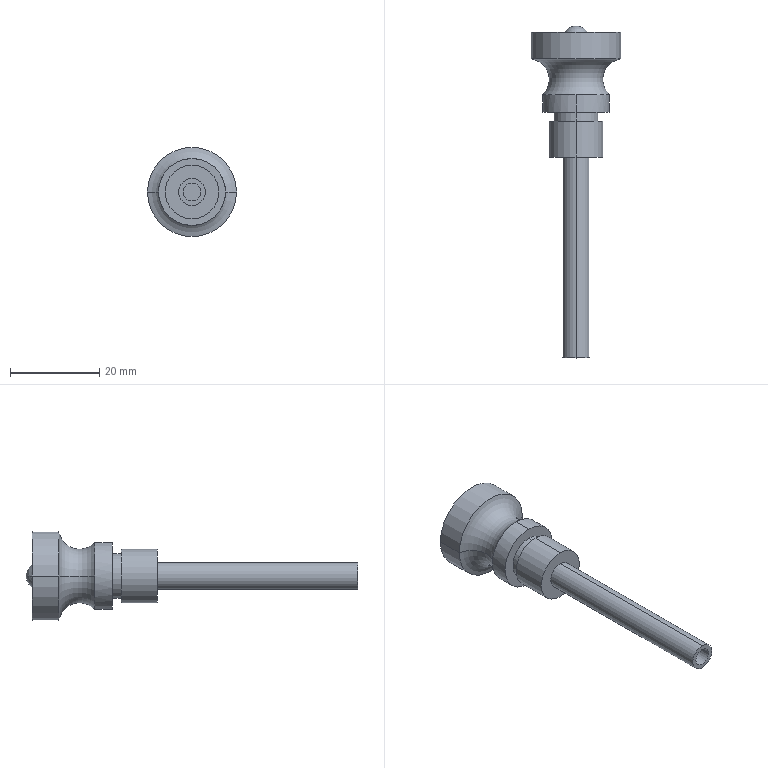Part | NX | features BREP 1 | 1 solid | 22 faces | box 20 x 74.367 x 20 mm | volume 5186 mm3 | cylinder 12 | plane 6 | torus 2 | sphere 2 | commonest cylinder face diameters 4 x2 6 x2 10 x2 12 x2 15 x2 20 x2
STEP:
#1=CARTESIAN_POINT('',(-10.,6.,0.));
#2=VERTEX_POINT('',#1);
#3=CARTESIAN_POINT('',(10.,6.,0.));
#4=VERTEX_POINT('',#3);
#5=CARTESIAN_POINT('',(0.,6.,0.));
#6=DIRECTION('',(0.,1.,0.));
#7=DIRECTION('',(-1.,0.,0.));
#8=AXIS2_PLACEMENT_3D('',#5,#6,#7);
#9=CIRCLE('',#8,10.);
#10=EDGE_CURVE('',#2,#4,#9,.T.);
#11=ORIENTED_EDGE('',*,*,#10,.T.);
#12=CARTESIAN_POINT('',(0.,6.,0.));
#13=DIRECTION('',(0.,1.,0.));
#14=DIRECTION('',(1.,0.,0.));
#15=AXIS2_PLACEMENT_3D('',#12,#13,#14);
#16=CIRCLE('',#15,10.);
#17=EDGE_CURVE('',#4,#2,#16,.T.);
#18=ORIENTED_EDGE('',*,*,#17,.T.);
#19=EDGE_LOOP('',(#11,#18));
#20=FACE_BOUND('',#19,.T.);
#21=CARTESIAN_POINT('',(-2.5,6.,0.));
#22=VERTEX_POINT('',#21);
#23=CARTESIAN_POINT('',(2.5,6.,0.));
#24=VERTEX_POINT('',#23);
#25=CARTESIAN_POINT('',(0.,6.,0.));
#26=DIRECTION('',(0.,-1.,0.));
#27=DIRECTION('',(-1.,0.,0.));
#28=AXIS2_PLACEMENT_3D('',#25,#26,#27);
#29=CIRCLE('',#28,2.5);
#30=EDGE_CURVE('',#22,#24,#29,.T.);
#31=ORIENTED_EDGE('',*,*,#30,.T.);
#32=CARTESIAN_POINT('',(0.,6.,0.));
#33=DIRECTION('',(0.,-1.,0.));
#34=DIRECTION('',(1.,0.,0.));
#35=AXIS2_PLACEMENT_3D('',#32,#33,#34);
#36=CIRCLE('',#35,2.5);
#37=EDGE_CURVE('',#24,#22,#36,.T.);
#38=ORIENTED_EDGE('',*,*,#37,.T.);
#39=EDGE_LOOP('',(#31,#38));
#40=FACE_BOUND('',#39,.T.);
#41=CARTESIAN_POINT('',(0.,6.,0.));
#42=DIRECTION('',(0.,1.,0.));
#43=DIRECTION('',(-1.,0.,0.));
#44=AXIS2_PLACEMENT_3D('',#41,#42,#43);
#45=PLANE('',#44);
#46=ADVANCED_FACE('',(#20,#40),#45,.T.);
#47=CARTESIAN_POINT('',(-10.,0.,0.));
#48=VERTEX_POINT('',#47);
#49=CARTESIAN_POINT('',(-10.,0.,0.));
#50=DIRECTION('',(0.,1.,0.));
#51=VECTOR('',#50,1000.);
#52=LINE('',#49,#51);
#53=EDGE_CURVE('',#48,#2,#52,.T.);
#54=ORIENTED_EDGE('',*,*,#53,.T.);
#55=ORIENTED_EDGE('',*,*,#17,.F.);
#56=CARTESIAN_POINT('',(10.,0.,0.));
#57=VERTEX_POINT('',#56);
#58=CARTESIAN_POINT('',(10.,0.,0.));
#59=DIRECTION('',(0.,1.,0.));
#60=VECTOR('',#59,1000.);
#61=LINE('',#58,#60);
#62=EDGE_CURVE('',#57,#4,#61,.T.);
#63=ORIENTED_EDGE('',*,*,#62,.F.);
#64=CARTESIAN_POINT('',(0.,0.,0.));
#65=DIRECTION('',(0.,-1.,0.));
#66=DIRECTION('',(-1.,0.,0.));
#67=AXIS2_PLACEMENT_3D('',#64,#65,#66);
#68=CIRCLE('',#67,10.);
#69=EDGE_CURVE('',#48,#57,#68,.T.);
#70=ORIENTED_EDGE('',*,*,#69,.F.);
#71=EDGE_LOOP('',(#54,#55,#63,#70));
#72=FACE_BOUND('',#71,.T.);
#73=CARTESIAN_POINT('',(0.,0.,0.));
#74=DIRECTION('',(0.,1.,0.));
#75=DIRECTION('',(-1.,0.,0.));
#76=AXIS2_PLACEMENT_3D('',#73,#74,#75);
#77=CYLINDRICAL_SURFACE('',#76,10.);
#78=ADVANCED_FACE('',(#72),#77,.T.);
#79=CARTESIAN_POINT('',(-7.5,-8.,0.));
#80=VERTEX_POINT('',#79);
#81=CARTESIAN_POINT('',(0.,-8.,-7.5));
#82=VERTEX_POINT('',#81);
#83=CARTESIAN_POINT('',(0.,-8.,0.));
#84=DIRECTION('',(0.,-1.,0.));
#85=DIRECTION('',(-1.,0.,0.));
#86=AXIS2_PLACEMENT_3D('',#83,#84,#85);
#87=CIRCLE('',#86,7.5);
#88=EDGE_CURVE('',#80,#82,#87,.T.);
#89=ORIENTED_EDGE('',*,*,#88,.F.);
#90=CARTESIAN_POINT('',(-10.631,-4.588,0.));
#91=DIRECTION('',(0.,0.,1.));
#92=DIRECTION('',(0.6761,-0.7368,0.));
#93=AXIS2_PLACEMENT_3D('',#90,#91,#92);
#94=CIRCLE('',#93,4.631);
#95=EDGE_CURVE('',#80,#48,#94,.T.);
#96=ORIENTED_EDGE('',*,*,#95,.T.);
#97=ORIENTED_EDGE('',*,*,#69,.T.);
#98=CARTESIAN_POINT('',(7.5,-8.,0.));
#99=VERTEX_POINT('',#98);
#100=CARTESIAN_POINT('',(10.631,-4.588,0.));
#101=DIRECTION('',(0.,0.,-1.));
#102=DIRECTION('',(-0.6761,-0.7368,0.));
#103=AXIS2_PLACEMENT_3D('',#100,#101,#102);
#104=CIRCLE('',#103,4.631);
#105=EDGE_CURVE('',#99,#57,#104,.T.);
#106=ORIENTED_EDGE('',*,*,#105,.F.);
#107=CARTESIAN_POINT('',(0.,-8.,0.));
#108=DIRECTION('',(0.,-1.,0.));
#109=DIRECTION('',(0.,0.,-1.));
#110=AXIS2_PLACEMENT_3D('',#107,#108,#109);
#111=CIRCLE('',#110,7.5);
#112=EDGE_CURVE('',#82,#99,#111,.T.);
#113=ORIENTED_EDGE('',*,*,#112,.F.);
#114=EDGE_LOOP('',(#89,#96,#97,#106,#113));
#115=FACE_BOUND('',#114,.T.);
#116=CARTESIAN_POINT('',(0.,-4.588,0.));
#117=DIRECTION('',(0.,-1.,0.));
#118=DIRECTION('',(1.,0.,0.));
#119=AXIS2_PLACEMENT_3D('',#116,#117,#118);
#120=TOROIDAL_SURFACE('',#119,10.631,4.631);
#121=ADVANCED_FACE('',(#115),#120,.F.);
#122=CARTESIAN_POINT('',(0.,-8.,7.5));
#123=VERTEX_POINT('',#122);
#124=CARTESIAN_POINT('',(0.,-8.,0.));
#125=DIRECTION('',(0.,-1.,0.));
#126=DIRECTION('',(1.,0.,0.));
#127=AXIS2_PLACEMENT_3D('',#124,#125,#126);
#128=CIRCLE('',#127,7.5);
#129=EDGE_CURVE('',#99,#123,#128,.T.);
#130=ORIENTED_EDGE('',*,*,#129,.T.);
#131=CARTESIAN_POINT('',(0.,-12.,7.5));
#132=VERTEX_POINT('',#131);
#133=CARTESIAN_POINT('',(0.,-8.,7.5));
#134=DIRECTION('',(0.,-1.,0.));
#135=VECTOR('',#134,1000.);
#136=LINE('',#133,#135);
#137=EDGE_CURVE('',#132,#123,#136,.F.);
#138=ORIENTED_EDGE('',*,*,#137,.F.);
#139=CARTESIAN_POINT('',(0.,-12.,-7.5));
#140=VERTEX_POINT('',#139);
#141=CARTESIAN_POINT('',(0.,-12.,0.));
#142=DIRECTION('',(0.,-1.,0.));
#143=DIRECTION('',(0.,0.,-1.));
#144=AXIS2_PLACEMENT_3D('',#141,#142,#143);
#145=CIRCLE('',#144,7.5);
#146=EDGE_CURVE('',#140,#132,#145,.T.);
#147=ORIENTED_EDGE('',*,*,#146,.F.);
#148=CARTESIAN_POINT('',(0.,-8.,-7.5));
#149=DIRECTION('',(0.,-1.,0.));
#150=VECTOR('',#149,1000.);
#151=LINE('',#148,#150);
#152=EDGE_CURVE('',#140,#82,#151,.F.);
#153=ORIENTED_EDGE('',*,*,#152,.T.);
#154=ORIENTED_EDGE('',*,*,#112,.T.);
#155=EDGE_LOOP('',(#130,#138,#147,#153,#154));
#156=FACE_BOUND('',#155,.T.);
#157=CARTESIAN_POINT('',(0.,-8.,0.));
#158=DIRECTION('',(0.,-1.,0.));
#159=DIRECTION('',(0.,0.,1.));
#160=AXIS2_PLACEMENT_3D('',#157,#158,#159);
#161=CYLINDRICAL_SURFACE('',#160,7.5);
#162=ADVANCED_FACE('',(#156),#161,.T.);
#163=ORIENTED_EDGE('',*,*,#88,.T.);
#164=ORIENTED_EDGE('',*,*,#152,.F.);
#165=CARTESIAN_POINT('',(0.,-12.,0.));
#166=DIRECTION('',(0.,-1.,0.));
#167=DIRECTION('',(0.,0.,1.));
#168=AXIS2_PLACEMENT_3D('',#165,#166,#167);
#169=CIRCLE('',#168,7.5);
#170=EDGE_CURVE('',#132,#140,#169,.T.);
#171=ORIENTED_EDGE('',*,*,#170,.F.);
#172=ORIENTED_EDGE('',*,*,#137,.T.);
#173=CARTESIAN_POINT('',(0.,-8.,0.));
#174=DIRECTION('',(0.,-1.,0.));
#175=DIRECTION('',(0.,0.,1.));
#176=AXIS2_PLACEMENT_3D('',#173,#174,#175);
#177=CIRCLE('',#176,7.5);
#178=EDGE_CURVE('',#123,#80,#177,.T.);
#179=ORIENTED_EDGE('',*,*,#178,.T.);
#180=EDGE_LOOP('',(#163,#164,#171,#172,#179));
#181=FACE_BOUND('',#180,.T.);
#182=CARTESIAN_POINT('',(0.,-8.,0.));
#183=DIRECTION('',(0.,-1.,0.));
#184=DIRECTION('',(0.,0.,1.));
#185=AXIS2_PLACEMENT_3D('',#182,#183,#184);
#186=CYLINDRICAL_SURFACE('',#185,7.5);
#187=ADVANCED_FACE('',(#181),#186,.T.);
#188=ORIENTED_EDGE('',*,*,#105,.T.);
#189=CARTESIAN_POINT('',(0.,0.,0.));
#190=DIRECTION('',(0.,-1.,0.));
#191=DIRECTION('',(1.,0.,0.));
#192=AXIS2_PLACEMENT_3D('',#189,#190,#191);
#193=CIRCLE('',#192,10.);
#194=EDGE_CURVE('',#57,#48,#193,.T.);
#195=ORIENTED_EDGE('',*,*,#194,.T.);
#196=ORIENTED_EDGE('',*,*,#95,.F.);
#197=ORIENTED_EDGE('',*,*,#178,.F.);
#198=ORIENTED_EDGE('',*,*,#129,.F.);
#199=EDGE_LOOP('',(#188,#195,#196,#197,#198));
#200=FACE_BOUND('',#199,.T.);
#201=CARTESIAN_POINT('',(0.,-4.588,0.));
#202=DIRECTION('',(0.,-1.,0.));
#203=DIRECTION('',(1.,0.,0.));
#204=AXIS2_PLACEMENT_3D('',#201,#202,#203);
#205=TOROIDAL_SURFACE('',#204,10.631,4.631);
#206=ADVANCED_FACE('',(#200),#205,.F.);
#207=ORIENTED_EDGE('',*,*,#62,.T.);
#208=ORIENTED_EDGE('',*,*,#10,.F.);
#209=ORIENTED_EDGE('',*,*,#53,.F.);
#210=ORIENTED_EDGE('',*,*,#194,.F.);
#211=EDGE_LOOP('',(#207,#208,#209,#210));
#212=FACE_BOUND('',#211,.T.);
#213=CARTESIAN_POINT('',(0.,0.,0.));
#214=DIRECTION('',(0.,1.,0.));
#215=DIRECTION('',(-1.,0.,0.));
#216=AXIS2_PLACEMENT_3D('',#213,#214,#215);
#217=CYLINDRICAL_SURFACE('',#216,10.);
#218=ADVANCED_FACE('',(#212),#217,.T.);
#219=ORIENTED_EDGE('',*,*,#170,.T.);
#220=ORIENTED_EDGE('',*,*,#146,.T.);
#221=EDGE_LOOP('',(#219,#220));
#222=FACE_BOUND('',#221,.T.);
#223=CARTESIAN_POINT('',(0.,-12.,5.));
#224=VERTEX_POINT('',#223);
#225=CARTESIAN_POINT('',(0.,-12.,-5.));
#226=VERTEX_POINT('',#225);
#227=CARTESIAN_POINT('',(0.,-12.,0.));
#228=DIRECTION('',(0.,-1.,0.));
#229=DIRECTION('',(0.,0.,1.));
#230=AXIS2_PLACEMENT_3D('',#227,#228,#229);
#231=CIRCLE('',#230,5.);
#232=EDGE_CURVE('',#224,#226,#231,.T.);
#233=ORIENTED_EDGE('',*,*,#232,.F.);
#234=CARTESIAN_POINT('',(0.,-12.,0.));
#235=DIRECTION('',(0.,-1.,0.));
#236=DIRECTION('',(0.,0.,-1.));
#237=AXIS2_PLACEMENT_3D('',#234,#235,#236);
#238=CIRCLE('',#237,5.);
#239=EDGE_CURVE('',#226,#224,#238,.T.);
#240=ORIENTED_EDGE('',*,*,#239,.F.);
#241=EDGE_LOOP('',(#233,#240));
#242=FACE_BOUND('',#241,.T.);
#243=CARTESIAN_POINT('',(0.,-12.,0.));
#244=DIRECTION('',(0.,-1.,0.));
#245=DIRECTION('',(0.,0.,1.));
#246=AXIS2_PLACEMENT_3D('',#243,#244,#245);
#247=PLANE('',#246);
#248=ADVANCED_FACE('',(#222,#242),#247,.T.);
#249=CARTESIAN_POINT('',(0.,-14.,-5.));
#250=VERTEX_POINT('',#249);
#251=CARTESIAN_POINT('',(0.,-12.,-5.));
#252=DIRECTION('',(0.,-1.,0.));
#253=VECTOR('',#252,1000.);
#254=LINE('',#251,#253);
#255=EDGE_CURVE('',#250,#226,#254,.F.);
#256=ORIENTED_EDGE('',*,*,#255,.T.);
#257=ORIENTED_EDGE('',*,*,#239,.T.);
#258=CARTESIAN_POINT('',(0.,-14.,5.));
#259=VERTEX_POINT('',#258);
#260=CARTESIAN_POINT('',(0.,-12.,5.));
#261=DIRECTION('',(0.,-1.,0.));
#262=VECTOR('',#261,1000.);
#263=LINE('',#260,#262);
#264=EDGE_CURVE('',#259,#224,#263,.F.);
#265=ORIENTED_EDGE('',*,*,#264,.F.);
#266=CARTESIAN_POINT('',(0.,-14.,0.));
#267=DIRECTION('',(0.,-1.,0.));
#268=DIRECTION('',(0.,0.,-1.));
#269=AXIS2_PLACEMENT_3D('',#266,#267,#268);
#270=CIRCLE('',#269,5.);
#271=EDGE_CURVE('',#250,#259,#270,.T.);
#272=ORIENTED_EDGE('',*,*,#271,.F.);
#273=EDGE_LOOP('',(#256,#257,#265,#272));
#274=FACE_BOUND('',#273,.T.);
#275=CARTESIAN_POINT('',(0.,-12.,0.));
#276=DIRECTION('',(0.,-1.,0.));
#277=DIRECTION('',(0.,0.,1.));
#278=AXIS2_PLACEMENT_3D('',#275,#276,#277);
#279=CYLINDRICAL_SURFACE('',#278,5.);
#280=ADVANCED_FACE('',(#274),#279,.T.);
#281=CARTESIAN_POINT('',(0.,-14.,6.));
#282=VERTEX_POINT('',#281);
#283=CARTESIAN_POINT('',(0.,-14.,-6.));
#284=VERTEX_POINT('',#283);
#285=CARTESIAN_POINT('',(0.,-14.,0.));
#286=DIRECTION('',(0.,-1.,0.));
#287=DIRECTION('',(0.,0.,1.));
#288=AXIS2_PLACEMENT_3D('',#285,#286,#287);
#289=CIRCLE('',#288,6.);
#290=EDGE_CURVE('',#282,#284,#289,.T.);
#291=ORIENTED_EDGE('',*,*,#290,.F.);
#292=CARTESIAN_POINT('',(0.,-14.,0.));
#293=DIRECTION('',(0.,-1.,0.));
#294=DIRECTION('',(0.,0.,-1.));
#295=AXIS2_PLACEMENT_3D('',#292,#293,#294);
#296=CIRCLE('',#295,6.);
#297=EDGE_CURVE('',#284,#282,#296,.T.);
#298=ORIENTED_EDGE('',*,*,#297,.F.);
#299=EDGE_LOOP('',(#291,#298));
#300=FACE_BOUND('',#299,.T.);
#301=CARTESIAN_POINT('',(0.,-14.,0.));
#302=DIRECTION('',(0.,-1.,0.));
#303=DIRECTION('',(0.,0.,1.));
#304=AXIS2_PLACEMENT_3D('',#301,#302,#303);
#305=CIRCLE('',#304,5.);
#306=EDGE_CURVE('',#259,#250,#305,.T.);
#307=ORIENTED_EDGE('',*,*,#306,.T.);
#308=ORIENTED_EDGE('',*,*,#271,.T.);
#309=EDGE_LOOP('',(#307,#308));
#310=FACE_BOUND('',#309,.T.);
#311=CARTESIAN_POINT('',(0.,-14.,0.));
#312=DIRECTION('',(0.,-1.,0.));
#313=DIRECTION('',(0.,0.,1.));
#314=AXIS2_PLACEMENT_3D('',#311,#312,#313);
#315=PLANE('',#314);
#316=ADVANCED_FACE('',(#300,#310),#315,.F.);
#317=CARTESIAN_POINT('',(0.,-22.,6.));
#318=VERTEX_POINT('',#317);
#319=CARTESIAN_POINT('',(0.,-14.,6.));
#320=DIRECTION('',(0.,-1.,0.));
#321=VECTOR('',#320,1000.);
#322=LINE('',#319,#321);
#323=EDGE_CURVE('',#318,#282,#322,.F.);
#324=ORIENTED_EDGE('',*,*,#323,.F.);
#325=CARTESIAN_POINT('',(0.,-22.,-6.));
#326=VERTEX_POINT('',#325);
#327=CARTESIAN_POINT('',(0.,-22.,0.));
#328=DIRECTION('',(0.,-1.,0.));
#329=DIRECTION('',(0.,0.,-1.));
#330=AXIS2_PLACEMENT_3D('',#327,#328,#329);
#331=CIRCLE('',#330,6.);
#332=EDGE_CURVE('',#326,#318,#331,.T.);
#333=ORIENTED_EDGE('',*,*,#332,.F.);
#334=CARTESIAN_POINT('',(0.,-14.,-6.));
#335=DIRECTION('',(0.,-1.,0.));
#336=VECTOR('',#335,1000.);
#337=LINE('',#334,#336);
#338=EDGE_CURVE('',#326,#284,#337,.F.);
#339=ORIENTED_EDGE('',*,*,#338,.T.);
#340=ORIENTED_EDGE('',*,*,#297,.T.);
#341=EDGE_LOOP('',(#324,#333,#339,#340));
#342=FACE_BOUND('',#341,.T.);
#343=CARTESIAN_POINT('',(0.,-14.,0.));
#344=DIRECTION('',(0.,-1.,0.));
#345=DIRECTION('',(0.,0.,1.));
#346=AXIS2_PLACEMENT_3D('',#343,#344,#345);
#347=CYLINDRICAL_SURFACE('',#346,6.);
#348=ADVANCED_FACE('',(#342),#347,.T.);
#349=ORIENTED_EDGE('',*,*,#338,.F.);
#350=CARTESIAN_POINT('',(0.,-22.,0.));
#351=DIRECTION('',(0.,-1.,0.));
#352=DIRECTION('',(0.,0.,1.));
#353=AXIS2_PLACEMENT_3D('',#350,#351,#352);
#354=CIRCLE('',#353,6.);
#355=EDGE_CURVE('',#318,#326,#354,.T.);
#356=ORIENTED_EDGE('',*,*,#355,.F.);
#357=ORIENTED_EDGE('',*,*,#323,.T.);
#358=ORIENTED_EDGE('',*,*,#290,.T.);
#359=EDGE_LOOP('',(#349,#356,#357,#358));
#360=FACE_BOUND('',#359,.T.);
#361=CARTESIAN_POINT('',(0.,-14.,0.));
#362=DIRECTION('',(0.,-1.,0.));
#363=DIRECTION('',(0.,0.,1.));
#364=AXIS2_PLACEMENT_3D('',#361,#362,#363);
#365=CYLINDRICAL_SURFACE('',#364,6.);
#366=ADVANCED_FACE('',(#360),#365,.T.);
#367=ORIENTED_EDGE('',*,*,#355,.T.);
#368=ORIENTED_EDGE('',*,*,#332,.T.);
#369=EDGE_LOOP('',(#367,#368));
#370=FACE_BOUND('',#369,.T.);
#371=CARTESIAN_POINT('',(0.,-22.,3.));
#372=VERTEX_POINT('',#371);
#373=CARTESIAN_POINT('',(0.,-22.,-3.));
#374=VERTEX_POINT('',#373);
#375=CARTESIAN_POINT('',(0.,-22.,0.));
#376=DIRECTION('',(0.,-1.,0.));
#377=DIRECTION('',(0.,0.,1.));
#378=AXIS2_PLACEMENT_3D('',#375,#376,#377);
#379=CIRCLE('',#378,3.);
#380=EDGE_CURVE('',#372,#374,#379,.T.);
#381=ORIENTED_EDGE('',*,*,#380,.F.);
#382=CARTESIAN_POINT('',(0.,-22.,0.));
#383=DIRECTION('',(0.,-1.,0.));
#384=DIRECTION('',(0.,0.,-1.));
#385=AXIS2_PLACEMENT_3D('',#382,#383,#384);
#386=CIRCLE('',#385,3.);
#387=EDGE_CURVE('',#374,#372,#386,.T.);
#388=ORIENTED_EDGE('',*,*,#387,.F.);
#389=EDGE_LOOP('',(#381,#388));
#390=FACE_BOUND('',#389,.T.);
#391=CARTESIAN_POINT('',(0.,-22.,0.));
#392=DIRECTION('',(0.,-1.,0.));
#393=DIRECTION('',(0.,0.,1.));
#394=AXIS2_PLACEMENT_3D('',#391,#392,#393);
#395=PLANE('',#394);
#396=ADVANCED_FACE('',(#370,#390),#395,.T.);
#397=CARTESIAN_POINT('',(0.,-67.,3.));
#398=VERTEX_POINT('',#397);
#399=CARTESIAN_POINT('',(0.,-22.,3.));
#400=DIRECTION('',(0.,-1.,0.));
#401=VECTOR('',#400,1000.);
#402=LINE('',#399,#401);
#403=EDGE_CURVE('',#398,#372,#402,.F.);
#404=ORIENTED_EDGE('',*,*,#403,.F.);
#405=CARTESIAN_POINT('',(0.,-67.,-3.));
#406=VERTEX_POINT('',#405);
#407=CARTESIAN_POINT('',(0.,-67.,0.));
#408=DIRECTION('',(0.,-1.,0.));
#409=DIRECTION('',(0.,0.,-1.));
#410=AXIS2_PLACEMENT_3D('',#407,#408,#409);
#411=CIRCLE('',#410,3.);
#412=EDGE_CURVE('',#406,#398,#411,.T.);
#413=ORIENTED_EDGE('',*,*,#412,.F.);
#414=CARTESIAN_POINT('',(0.,-22.,-3.));
#415=DIRECTION('',(0.,-1.,0.));
#416=VECTOR('',#415,1000.);
#417=LINE('',#414,#416);
#418=EDGE_CURVE('',#406,#374,#417,.F.);
#419=ORIENTED_EDGE('',*,*,#418,.T.);
#420=ORIENTED_EDGE('',*,*,#387,.T.);
#421=EDGE_LOOP('',(#404,#413,#419,#420));
#422=FACE_BOUND('',#421,.T.);
#423=CARTESIAN_POINT('',(0.,-22.,0.));
#424=DIRECTION('',(0.,-1.,0.));
#425=DIRECTION('',(0.,0.,1.));
#426=AXIS2_PLACEMENT_3D('',#423,#424,#425);
#427=CYLINDRICAL_SURFACE('',#426,3.);
#428=ADVANCED_FACE('',(#422),#427,.T.);
#429=ORIENTED_EDGE('',*,*,#418,.F.);
#430=CARTESIAN_POINT('',(0.,-67.,0.));
#431=DIRECTION('',(0.,-1.,0.));
#432=DIRECTION('',(0.,0.,1.));
#433=AXIS2_PLACEMENT_3D('',#430,#431,#432);
#434=CIRCLE('',#433,3.);
#435=EDGE_CURVE('',#398,#406,#434,.T.);
#436=ORIENTED_EDGE('',*,*,#435,.F.);
#437=ORIENTED_EDGE('',*,*,#403,.T.);
#438=ORIENTED_EDGE('',*,*,#380,.T.);
#439=EDGE_LOOP('',(#429,#436,#437,#438));
#440=FACE_BOUND('',#439,.T.);
#441=CARTESIAN_POINT('',(0.,-22.,0.));
#442=DIRECTION('',(0.,-1.,0.));
#443=DIRECTION('',(0.,0.,1.));
#444=AXIS2_PLACEMENT_3D('',#441,#442,#443);
#445=CYLINDRICAL_SURFACE('',#444,3.);
#446=ADVANCED_FACE('',(#440),#445,.T.);
#447=ORIENTED_EDGE('',*,*,#435,.T.);
#448=ORIENTED_EDGE('',*,*,#412,.T.);
#449=EDGE_LOOP('',(#447,#448));
#450=FACE_BOUND('',#449,.T.);
#451=CARTESIAN_POINT('',(2.,-67.,0.));
#452=VERTEX_POINT('',#451);
#453=CARTESIAN_POINT('',(-2.,-67.,0.));
#454=VERTEX_POINT('',#453);
#455=CARTESIAN_POINT('',(0.,-67.,0.));
#456=DIRECTION('',(0.,1.,0.));
#457=DIRECTION('',(1.,0.,0.));
#458=AXIS2_PLACEMENT_3D('',#455,#456,#457);
#459=CIRCLE('',#458,2.);
#460=EDGE_CURVE('',#452,#454,#459,.T.);
#461=ORIENTED_EDGE('',*,*,#460,.T.);
#462=CARTESIAN_POINT('',(0.,-67.,0.));
#463=DIRECTION('',(0.,1.,0.));
#464=DIRECTION('',(-1.,0.,0.));
#465=AXIS2_PLACEMENT_3D('',#462,#463,#464);
#466=CIRCLE('',#465,2.);
#467=EDGE_CURVE('',#454,#452,#466,.T.);
#468=ORIENTED_EDGE('',*,*,#467,.T.);
#469=EDGE_LOOP('',(#461,#468));
#470=FACE_BOUND('',#469,.T.);
#471=CARTESIAN_POINT('',(0.,-67.,0.));
#472=DIRECTION('',(0.,-1.,0.));
#473=DIRECTION('',(0.,0.,1.));
#474=AXIS2_PLACEMENT_3D('',#471,#472,#473);
#475=PLANE('',#474);
#476=ADVANCED_FACE('',(#450,#470),#475,.T.);
#477=CARTESIAN_POINT('',(2.,6.,0.));
#478=VERTEX_POINT('',#477);
#479=CARTESIAN_POINT('',(2.,-67.,0.));
#480=DIRECTION('',(0.,1.,0.));
#481=VECTOR('',#480,1000.);
#482=LINE('',#479,#481);
#483=EDGE_CURVE('',#452,#478,#482,.T.);
#484=ORIENTED_EDGE('',*,*,#483,.F.);
#485=ORIENTED_EDGE('',*,*,#467,.F.);
#486=CARTESIAN_POINT('',(-2.,6.,0.));
#487=VERTEX_POINT('',#486);
#488=CARTESIAN_POINT('',(-2.,-67.,0.));
#489=DIRECTION('',(0.,1.,0.));
#490=VECTOR('',#489,1000.);
#491=LINE('',#488,#490);
#492=EDGE_CURVE('',#454,#487,#491,.T.);
#493=ORIENTED_EDGE('',*,*,#492,.T.);
#494=CARTESIAN_POINT('',(0.,6.,0.));
#495=DIRECTION('',(0.,1.,0.));
#496=DIRECTION('',(-1.,0.,0.));
#497=AXIS2_PLACEMENT_3D('',#494,#495,#496);
#498=CIRCLE('',#497,2.);
#499=EDGE_CURVE('',#487,#478,#498,.T.);
#500=ORIENTED_EDGE('',*,*,#499,.T.);
#501=EDGE_LOOP('',(#484,#485,#493,#500));
#502=FACE_BOUND('',#501,.T.);
#503=CARTESIAN_POINT('',(0.,-67.,0.));
#504=DIRECTION('',(0.,1.,0.));
#505=DIRECTION('',(1.,0.,0.));
#506=AXIS2_PLACEMENT_3D('',#503,#504,#505);
#507=CYLINDRICAL_SURFACE('',#506,2.);
#508=ADVANCED_FACE('',(#502),#507,.F.);
#509=CARTESIAN_POINT('',(0.,6.,0.));
#510=DIRECTION('',(0.,1.,0.));
#511=DIRECTION('',(1.,0.,0.));
#512=AXIS2_PLACEMENT_3D('',#509,#510,#511);
#513=CIRCLE('',#512,2.);
#514=EDGE_CURVE('',#478,#487,#513,.T.);
#515=ORIENTED_EDGE('',*,*,#514,.F.);
#516=ORIENTED_EDGE('',*,*,#499,.F.);
#517=EDGE_LOOP('',(#515,#516));
#518=FACE_BOUND('',#517,.T.);
#519=CARTESIAN_POINT('',(0.,6.,0.));
#520=DIRECTION('',(0.,-1.,0.));
#521=DIRECTION('',(1.,0.,0.));
#522=AXIS2_PLACEMENT_3D('',#519,#520,#521);
#523=PLANE('',#522);
#524=ADVANCED_FACE('',(#518),#523,.T.);
#525=ORIENTED_EDGE('',*,*,#492,.F.);
#526=ORIENTED_EDGE('',*,*,#460,.F.);
#527=ORIENTED_EDGE('',*,*,#483,.T.);
#528=ORIENTED_EDGE('',*,*,#514,.T.);
#529=EDGE_LOOP('',(#525,#526,#527,#528));
#530=FACE_BOUND('',#529,.T.);
#531=CARTESIAN_POINT('',(0.,-67.,0.));
#532=DIRECTION('',(0.,1.,0.));
#533=DIRECTION('',(1.,0.,0.));
#534=AXIS2_PLACEMENT_3D('',#531,#532,#533);
#535=CYLINDRICAL_SURFACE('',#534,2.);
#536=ADVANCED_FACE('',(#530),#535,.F.);
#537=ORIENTED_EDGE('',*,*,#264,.T.);
#538=ORIENTED_EDGE('',*,*,#232,.T.);
#539=ORIENTED_EDGE('',*,*,#255,.F.);
#540=ORIENTED_EDGE('',*,*,#306,.F.);
#541=EDGE_LOOP('',(#537,#538,#539,#540));
#542=FACE_BOUND('',#541,.T.);
#543=CARTESIAN_POINT('',(0.,-12.,0.));
#544=DIRECTION('',(0.,-1.,0.));
#545=DIRECTION('',(0.,0.,1.));
#546=AXIS2_PLACEMENT_3D('',#543,#544,#545);
#547=CYLINDRICAL_SURFACE('',#546,5.);
#548=ADVANCED_FACE('',(#542),#547,.T.);
#549=CARTESIAN_POINT('',(0.,7.367,0.));
#550=VERTEX_POINT('',#549);
#551=CARTESIAN_POINT('',(0.,4.398,0.));
#552=DIRECTION('',(0.,0.,1.));
#553=DIRECTION('',(0.8419,0.5396,0.));
#554=AXIS2_PLACEMENT_3D('',#551,#552,#553);
#555=CIRCLE('',#554,2.969);
#556=EDGE_CURVE('',#550,#24,#555,.F.);
#557=ORIENTED_EDGE('',*,*,#556,.F.);
#558=CARTESIAN_POINT('',(0.,4.398,0.));
#559=DIRECTION('',(0.,0.,-1.));
#560=DIRECTION('',(-0.8419,0.5396,0.));
#561=AXIS2_PLACEMENT_3D('',#558,#559,#560);
#562=CIRCLE('',#561,2.969);
#563=EDGE_CURVE('',#550,#22,#562,.F.);
#564=ORIENTED_EDGE('',*,*,#563,.T.);
#565=ORIENTED_EDGE('',*,*,#37,.F.);
#566=EDGE_LOOP('',(#557,#564,#565));
#567=FACE_BOUND('',#566,.T.);
#568=CARTESIAN_POINT('',(0.,4.398,0.));
#569=DIRECTION('',(0.,-1.,0.));
#570=DIRECTION('',(1.,0.,0.));
#571=AXIS2_PLACEMENT_3D('',#568,#569,#570);
#572=SPHERICAL_SURFACE('',#571,2.969);
#573=ADVANCED_FACE('',(#567),#572,.T.);
#574=ORIENTED_EDGE('',*,*,#563,.F.);
#575=ORIENTED_EDGE('',*,*,#556,.T.);
#576=ORIENTED_EDGE('',*,*,#30,.F.);
#577=EDGE_LOOP('',(#574,#575,#576));
#578=FACE_BOUND('',#577,.T.);
#579=CARTESIAN_POINT('',(0.,4.398,0.));
#580=DIRECTION('',(0.,-1.,0.));
#581=DIRECTION('',(1.,0.,0.));
#582=AXIS2_PLACEMENT_3D('',#579,#580,#581);
#583=SPHERICAL_SURFACE('',#582,2.969);
#584=ADVANCED_FACE('',(#578),#583,.T.);
#585=CLOSED_SHELL('',(#46,#78,#121,#162,#187,#206,#218,#248,#280,#316,#348,#366,#396,#428,#446,#476,#508,#524,#536,#548,#573,#584));
#586=MANIFOLD_SOLID_BREP('',#585);
#587=(LENGTH_UNIT()NAMED_UNIT(*)SI_UNIT(.MILLI.,.METRE.));
#588=UNCERTAINTY_MEASURE_WITH_UNIT(LENGTH_MEASURE(0.00001),#587,'','');
#589=(NAMED_UNIT(*)PLANE_ANGLE_UNIT()SI_UNIT($,.RADIAN.));
#590=(NAMED_UNIT(*)SI_UNIT($,.STERADIAN.)SOLID_ANGLE_UNIT());
#591=(GEOMETRIC_REPRESENTATION_CONTEXT(3)GLOBAL_UNCERTAINTY_ASSIGNED_CONTEXT((#588))GLOBAL_UNIT_ASSIGNED_CONTEXT((#587,#589,#590))REPRESENTATION_CONTEXT('',''));
#592=ADVANCED_BREP_SHAPE_REPRESENTATION('',(#586),#591);